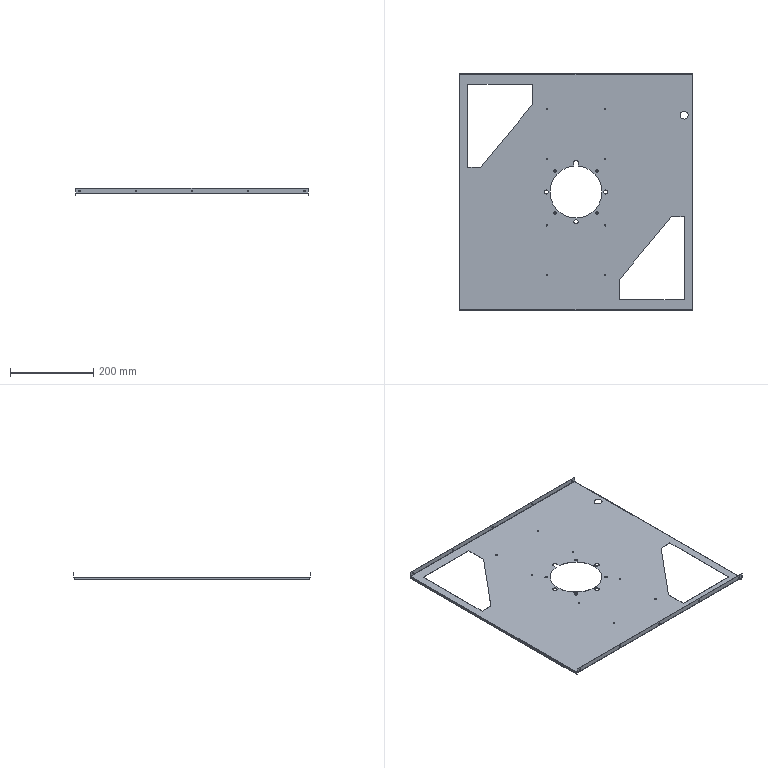Part | SolidWorks | features BaseBody 1 | 1 solid | 102 faces | box 560 x 568.8 x 17.4 mm | volume 168286 mm3 | cylinder 64 | plane 38 | commonest cylinder face diameters 3.5 x36 6.1 x8 10 x7 0.4 x4 1.6 x4 125 x3